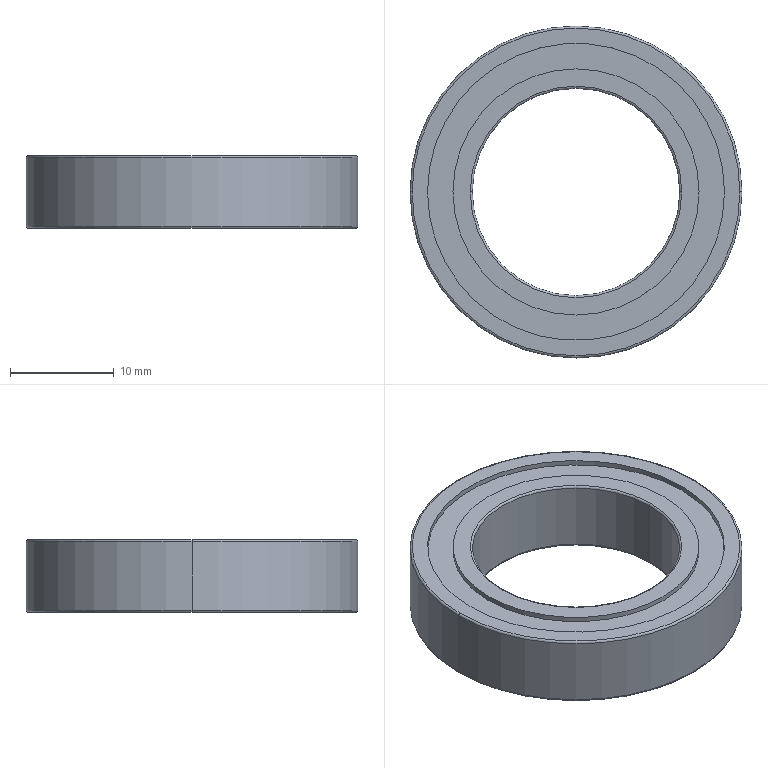Part | NX | features BREP 1 | 1 solid | 26 faces | box 32 x 32 x 7 mm | volume 3226 mm3 | cylinder 12 | torus 8 | plane 6 | commonest cylinder face diameters 23.732 x4 28.634 x4 20 x2 32 x2
STEP:
#1=CARTESIAN_POINT('',(-14.317,0.,3.));
#2=VERTEX_POINT('',#1);
#3=CARTESIAN_POINT('',(-14.317,0.,3.5));
#4=VERTEX_POINT('',#3);
#5=CARTESIAN_POINT('',(-14.317,0.,3.5));
#6=DIRECTION('',(0.,0.,-1.));
#7=VECTOR('',#6,1000.);
#8=LINE('',#5,#7);
#9=EDGE_CURVE('',#2,#4,#8,.F.);
#10=ORIENTED_EDGE('',*,*,#9,.T.);
#11=CARTESIAN_POINT('',(14.317,0.,3.5));
#12=VERTEX_POINT('',#11);
#13=CARTESIAN_POINT('',(0.,0.,3.5));
#14=DIRECTION('',(0.,0.,-1.));
#15=DIRECTION('',(1.,0.,0.));
#16=AXIS2_PLACEMENT_3D('',#13,#14,#15);
#17=CIRCLE('',#16,14.317);
#18=EDGE_CURVE('',#12,#4,#17,.T.);
#19=ORIENTED_EDGE('',*,*,#18,.F.);
#20=CARTESIAN_POINT('',(14.317,0.,3.));
#21=VERTEX_POINT('',#20);
#22=CARTESIAN_POINT('',(14.317,0.,3.5));
#23=DIRECTION('',(0.,0.,-1.));
#24=VECTOR('',#23,1000.);
#25=LINE('',#22,#24);
#26=EDGE_CURVE('',#21,#12,#25,.F.);
#27=ORIENTED_EDGE('',*,*,#26,.F.);
#28=CARTESIAN_POINT('',(0.,0.,3.));
#29=DIRECTION('',(0.,0.,1.));
#30=DIRECTION('',(-1.,0.,0.));
#31=AXIS2_PLACEMENT_3D('',#28,#29,#30);
#32=CIRCLE('',#31,14.317);
#33=EDGE_CURVE('',#2,#21,#32,.T.);
#34=ORIENTED_EDGE('',*,*,#33,.F.);
#35=EDGE_LOOP('',(#10,#19,#27,#34));
#36=FACE_BOUND('',#35,.T.);
#37=CARTESIAN_POINT('',(0.,0.,3.));
#38=DIRECTION('',(0.,0.,1.));
#39=DIRECTION('',(-1.,0.,0.));
#40=AXIS2_PLACEMENT_3D('',#37,#38,#39);
#41=CYLINDRICAL_SURFACE('',#40,14.317);
#42=ADVANCED_FACE('',(#36),#41,.F.);
#43=ORIENTED_EDGE('',*,*,#33,.T.);
#44=CARTESIAN_POINT('',(0.,0.,3.));
#45=DIRECTION('',(0.,0.,1.));
#46=DIRECTION('',(1.,0.,0.));
#47=AXIS2_PLACEMENT_3D('',#44,#45,#46);
#48=CIRCLE('',#47,14.317);
#49=EDGE_CURVE('',#21,#2,#48,.T.);
#50=ORIENTED_EDGE('',*,*,#49,.T.);
#51=EDGE_LOOP('',(#43,#50));
#52=FACE_BOUND('',#51,.T.);
#53=CARTESIAN_POINT('',(11.866,0.,3.));
#54=VERTEX_POINT('',#53);
#55=CARTESIAN_POINT('',(-11.866,0.,3.));
#56=VERTEX_POINT('',#55);
#57=CARTESIAN_POINT('',(0.,0.,3.));
#58=DIRECTION('',(0.,0.,-1.));
#59=DIRECTION('',(1.,0.,0.));
#60=AXIS2_PLACEMENT_3D('',#57,#58,#59);
#61=CIRCLE('',#60,11.866);
#62=EDGE_CURVE('',#54,#56,#61,.T.);
#63=ORIENTED_EDGE('',*,*,#62,.T.);
#64=CARTESIAN_POINT('',(0.,0.,3.));
#65=DIRECTION('',(0.,0.,-1.));
#66=DIRECTION('',(-1.,0.,0.));
#67=AXIS2_PLACEMENT_3D('',#64,#65,#66);
#68=CIRCLE('',#67,11.866);
#69=EDGE_CURVE('',#56,#54,#68,.T.);
#70=ORIENTED_EDGE('',*,*,#69,.T.);
#71=EDGE_LOOP('',(#63,#70));
#72=FACE_BOUND('',#71,.T.);
#73=CARTESIAN_POINT('',(0.,0.,3.));
#74=DIRECTION('',(0.,0.,1.));
#75=DIRECTION('',(-1.,0.,0.));
#76=AXIS2_PLACEMENT_3D('',#73,#74,#75);
#77=PLANE('',#76);
#78=ADVANCED_FACE('',(#52,#72),#77,.T.);
#79=ORIENTED_EDGE('',*,*,#49,.F.);
#80=ORIENTED_EDGE('',*,*,#26,.T.);
#81=CARTESIAN_POINT('',(0.,0.,3.5));
#82=DIRECTION('',(0.,0.,-1.));
#83=DIRECTION('',(-1.,0.,0.));
#84=AXIS2_PLACEMENT_3D('',#81,#82,#83);
#85=CIRCLE('',#84,14.317);
#86=EDGE_CURVE('',#4,#12,#85,.T.);
#87=ORIENTED_EDGE('',*,*,#86,.F.);
#88=ORIENTED_EDGE('',*,*,#9,.F.);
#89=EDGE_LOOP('',(#79,#80,#87,#88));
#90=FACE_BOUND('',#89,.T.);
#91=CARTESIAN_POINT('',(0.,0.,3.));
#92=DIRECTION('',(0.,0.,1.));
#93=DIRECTION('',(-1.,0.,0.));
#94=AXIS2_PLACEMENT_3D('',#91,#92,#93);
#95=CYLINDRICAL_SURFACE('',#94,14.317);
#96=ADVANCED_FACE('',(#90),#95,.F.);
#97=CARTESIAN_POINT('',(-15.8,0.,3.5));
#98=VERTEX_POINT('',#97);
#99=CARTESIAN_POINT('',(15.8,0.,3.5));
#100=VERTEX_POINT('',#99);
#101=CARTESIAN_POINT('',(0.,0.,3.5));
#102=DIRECTION('',(0.,0.,1.));
#103=DIRECTION('',(-1.,0.,0.));
#104=AXIS2_PLACEMENT_3D('',#101,#102,#103);
#105=CIRCLE('',#104,15.8);
#106=EDGE_CURVE('',#98,#100,#105,.T.);
#107=ORIENTED_EDGE('',*,*,#106,.T.);
#108=CARTESIAN_POINT('',(0.,0.,3.5));
#109=DIRECTION('',(0.,0.,1.));
#110=DIRECTION('',(1.,0.,0.));
#111=AXIS2_PLACEMENT_3D('',#108,#109,#110);
#112=CIRCLE('',#111,15.8);
#113=EDGE_CURVE('',#100,#98,#112,.T.);
#114=ORIENTED_EDGE('',*,*,#113,.T.);
#115=EDGE_LOOP('',(#107,#114));
#116=FACE_BOUND('',#115,.T.);
#117=ORIENTED_EDGE('',*,*,#18,.T.);
#118=ORIENTED_EDGE('',*,*,#86,.T.);
#119=EDGE_LOOP('',(#117,#118));
#120=FACE_BOUND('',#119,.T.);
#121=CARTESIAN_POINT('',(0.,0.,3.5));
#122=DIRECTION('',(0.,0.,1.));
#123=DIRECTION('',(-1.,0.,0.));
#124=AXIS2_PLACEMENT_3D('',#121,#122,#123);
#125=PLANE('',#124);
#126=ADVANCED_FACE('',(#116,#120),#125,.T.);
#127=CARTESIAN_POINT('',(-16.,0.,3.3));
#128=VERTEX_POINT('',#127);
#129=CARTESIAN_POINT('',(-15.8,0.,3.3));
#130=DIRECTION('',(0.,-1.,0.));
#131=DIRECTION('',(0.,0.,1.));
#132=AXIS2_PLACEMENT_3D('',#129,#130,#131);
#133=CIRCLE('',#132,0.2);
#134=EDGE_CURVE('',#128,#98,#133,.F.);
#135=ORIENTED_EDGE('',*,*,#134,.T.);
#136=ORIENTED_EDGE('',*,*,#113,.F.);
#137=CARTESIAN_POINT('',(16.,0.,3.3));
#138=VERTEX_POINT('',#137);
#139=CARTESIAN_POINT('',(15.8,0.,3.3));
#140=DIRECTION('',(0.,1.,0.));
#141=DIRECTION('',(0.,0.,1.));
#142=AXIS2_PLACEMENT_3D('',#139,#140,#141);
#143=CIRCLE('',#142,0.2);
#144=EDGE_CURVE('',#138,#100,#143,.F.);
#145=ORIENTED_EDGE('',*,*,#144,.F.);
#146=CARTESIAN_POINT('',(0.,0.,3.3));
#147=DIRECTION('',(0.,0.,1.));
#148=DIRECTION('',(1.,0.,0.));
#149=AXIS2_PLACEMENT_3D('',#146,#147,#148);
#150=CIRCLE('',#149,16.);
#151=EDGE_CURVE('',#138,#128,#150,.T.);
#152=ORIENTED_EDGE('',*,*,#151,.T.);
#153=EDGE_LOOP('',(#135,#136,#145,#152));
#154=FACE_BOUND('',#153,.T.);
#155=CARTESIAN_POINT('',(0.,0.,3.3));
#156=DIRECTION('',(0.,0.,1.));
#157=DIRECTION('',(-1.,0.,0.));
#158=AXIS2_PLACEMENT_3D('',#155,#156,#157);
#159=TOROIDAL_SURFACE('',#158,15.8,0.2);
#160=ADVANCED_FACE('',(#154),#159,.T.);
#161=CARTESIAN_POINT('',(16.,0.,-3.3));
#162=VERTEX_POINT('',#161);
#163=CARTESIAN_POINT('',(16.,0.,-3.3));
#164=DIRECTION('',(0.,0.,1.));
#165=VECTOR('',#164,1000.);
#166=LINE('',#163,#165);
#167=EDGE_CURVE('',#162,#138,#166,.T.);
#168=ORIENTED_EDGE('',*,*,#167,.F.);
#169=CARTESIAN_POINT('',(-16.,0.,-3.3));
#170=VERTEX_POINT('',#169);
#171=CARTESIAN_POINT('',(0.,0.,-3.3));
#172=DIRECTION('',(0.,0.,-1.));
#173=DIRECTION('',(-1.,0.,0.));
#174=AXIS2_PLACEMENT_3D('',#171,#172,#173);
#175=CIRCLE('',#174,16.);
#176=EDGE_CURVE('',#170,#162,#175,.T.);
#177=ORIENTED_EDGE('',*,*,#176,.F.);
#178=CARTESIAN_POINT('',(-16.,0.,-3.3));
#179=DIRECTION('',(0.,0.,1.));
#180=VECTOR('',#179,1000.);
#181=LINE('',#178,#180);
#182=EDGE_CURVE('',#170,#128,#181,.T.);
#183=ORIENTED_EDGE('',*,*,#182,.T.);
#184=ORIENTED_EDGE('',*,*,#151,.F.);
#185=EDGE_LOOP('',(#168,#177,#183,#184));
#186=FACE_BOUND('',#185,.T.);
#187=CARTESIAN_POINT('',(0.,0.,3.5));
#188=DIRECTION('',(0.,0.,-1.));
#189=DIRECTION('',(1.,0.,0.));
#190=AXIS2_PLACEMENT_3D('',#187,#188,#189);
#191=CYLINDRICAL_SURFACE('',#190,16.);
#192=ADVANCED_FACE('',(#186),#191,.T.);
#193=CARTESIAN_POINT('',(0.,0.,3.3));
#194=DIRECTION('',(0.,0.,1.));
#195=DIRECTION('',(-1.,0.,0.));
#196=AXIS2_PLACEMENT_3D('',#193,#194,#195);
#197=CIRCLE('',#196,16.);
#198=EDGE_CURVE('',#128,#138,#197,.T.);
#199=ORIENTED_EDGE('',*,*,#198,.F.);
#200=ORIENTED_EDGE('',*,*,#182,.F.);
#201=CARTESIAN_POINT('',(0.,0.,-3.3));
#202=DIRECTION('',(0.,0.,-1.));
#203=DIRECTION('',(1.,0.,0.));
#204=AXIS2_PLACEMENT_3D('',#201,#202,#203);
#205=CIRCLE('',#204,16.);
#206=EDGE_CURVE('',#162,#170,#205,.T.);
#207=ORIENTED_EDGE('',*,*,#206,.F.);
#208=ORIENTED_EDGE('',*,*,#167,.T.);
#209=EDGE_LOOP('',(#199,#200,#207,#208));
#210=FACE_BOUND('',#209,.T.);
#211=CARTESIAN_POINT('',(0.,0.,3.5));
#212=DIRECTION('',(0.,0.,-1.));
#213=DIRECTION('',(1.,0.,0.));
#214=AXIS2_PLACEMENT_3D('',#211,#212,#213);
#215=CYLINDRICAL_SURFACE('',#214,16.);
#216=ADVANCED_FACE('',(#210),#215,.T.);
#217=CARTESIAN_POINT('',(15.8,0.,-3.5));
#218=VERTEX_POINT('',#217);
#219=CARTESIAN_POINT('',(-15.8,0.,-3.5));
#220=VERTEX_POINT('',#219);
#221=CARTESIAN_POINT('',(0.,0.,-3.5));
#222=DIRECTION('',(0.,0.,-1.));
#223=DIRECTION('',(1.,0.,0.));
#224=AXIS2_PLACEMENT_3D('',#221,#222,#223);
#225=CIRCLE('',#224,15.8);
#226=EDGE_CURVE('',#218,#220,#225,.T.);
#227=ORIENTED_EDGE('',*,*,#226,.F.);
#228=CARTESIAN_POINT('',(15.8,0.,-3.3));
#229=DIRECTION('',(0.,1.,0.));
#230=DIRECTION('',(1.,0.,0.));
#231=AXIS2_PLACEMENT_3D('',#228,#229,#230);
#232=CIRCLE('',#231,0.2);
#233=EDGE_CURVE('',#162,#218,#232,.T.);
#234=ORIENTED_EDGE('',*,*,#233,.F.);
#235=ORIENTED_EDGE('',*,*,#206,.T.);
#236=CARTESIAN_POINT('',(-15.8,0.,-3.3));
#237=DIRECTION('',(0.,-1.,0.));
#238=DIRECTION('',(-1.,0.,0.));
#239=AXIS2_PLACEMENT_3D('',#236,#237,#238);
#240=CIRCLE('',#239,0.2);
#241=EDGE_CURVE('',#170,#220,#240,.T.);
#242=ORIENTED_EDGE('',*,*,#241,.T.);
#243=EDGE_LOOP('',(#227,#234,#235,#242));
#244=FACE_BOUND('',#243,.T.);
#245=CARTESIAN_POINT('',(0.,0.,-3.3));
#246=DIRECTION('',(0.,0.,1.));
#247=DIRECTION('',(-1.,0.,0.));
#248=AXIS2_PLACEMENT_3D('',#245,#246,#247);
#249=TOROIDAL_SURFACE('',#248,15.8,0.2);
#250=ADVANCED_FACE('',(#244),#249,.T.);
#251=ORIENTED_EDGE('',*,*,#241,.F.);
#252=ORIENTED_EDGE('',*,*,#176,.T.);
#253=ORIENTED_EDGE('',*,*,#233,.T.);
#254=CARTESIAN_POINT('',(0.,0.,-3.5));
#255=DIRECTION('',(0.,0.,-1.));
#256=DIRECTION('',(-1.,0.,0.));
#257=AXIS2_PLACEMENT_3D('',#254,#255,#256);
#258=CIRCLE('',#257,15.8);
#259=EDGE_CURVE('',#220,#218,#258,.T.);
#260=ORIENTED_EDGE('',*,*,#259,.F.);
#261=EDGE_LOOP('',(#251,#252,#253,#260));
#262=FACE_BOUND('',#261,.T.);
#263=CARTESIAN_POINT('',(0.,0.,-3.3));
#264=DIRECTION('',(0.,0.,1.));
#265=DIRECTION('',(-1.,0.,0.));
#266=AXIS2_PLACEMENT_3D('',#263,#264,#265);
#267=TOROIDAL_SURFACE('',#266,15.8,0.2);
#268=ADVANCED_FACE('',(#262),#267,.T.);
#269=ORIENTED_EDGE('',*,*,#259,.T.);
#270=ORIENTED_EDGE('',*,*,#226,.T.);
#271=EDGE_LOOP('',(#269,#270));
#272=FACE_BOUND('',#271,.T.);
#273=CARTESIAN_POINT('',(14.317,0.,-3.5));
#274=VERTEX_POINT('',#273);
#275=CARTESIAN_POINT('',(-14.317,0.,-3.5));
#276=VERTEX_POINT('',#275);
#277=CARTESIAN_POINT('',(0.,0.,-3.5));
#278=DIRECTION('',(0.,0.,1.));
#279=DIRECTION('',(1.,0.,0.));
#280=AXIS2_PLACEMENT_3D('',#277,#278,#279);
#281=CIRCLE('',#280,14.317);
#282=EDGE_CURVE('',#274,#276,#281,.T.);
#283=ORIENTED_EDGE('',*,*,#282,.T.);
#284=CARTESIAN_POINT('',(0.,0.,-3.5));
#285=DIRECTION('',(0.,0.,1.));
#286=DIRECTION('',(-1.,0.,0.));
#287=AXIS2_PLACEMENT_3D('',#284,#285,#286);
#288=CIRCLE('',#287,14.317);
#289=EDGE_CURVE('',#276,#274,#288,.T.);
#290=ORIENTED_EDGE('',*,*,#289,.T.);
#291=EDGE_LOOP('',(#283,#290));
#292=FACE_BOUND('',#291,.T.);
#293=CARTESIAN_POINT('',(0.,0.,-3.5));
#294=DIRECTION('',(0.,0.,1.));
#295=DIRECTION('',(-1.,0.,0.));
#296=AXIS2_PLACEMENT_3D('',#293,#294,#295);
#297=PLANE('',#296);
#298=ADVANCED_FACE('',(#272,#292),#297,.F.);
#299=CARTESIAN_POINT('',(14.317,0.,-3.));
#300=VERTEX_POINT('',#299);
#301=CARTESIAN_POINT('',(14.317,0.,-3.5));
#302=DIRECTION('',(0.,0.,1.));
#303=VECTOR('',#302,1000.);
#304=LINE('',#301,#303);
#305=EDGE_CURVE('',#274,#300,#304,.T.);
#306=ORIENTED_EDGE('',*,*,#305,.F.);
#307=ORIENTED_EDGE('',*,*,#289,.F.);
#308=CARTESIAN_POINT('',(-14.317,0.,-3.));
#309=VERTEX_POINT('',#308);
#310=CARTESIAN_POINT('',(-14.317,0.,-3.5));
#311=DIRECTION('',(0.,0.,1.));
#312=VECTOR('',#311,1000.);
#313=LINE('',#310,#312);
#314=EDGE_CURVE('',#276,#309,#313,.T.);
#315=ORIENTED_EDGE('',*,*,#314,.T.);
#316=CARTESIAN_POINT('',(0.,0.,-3.));
#317=DIRECTION('',(0.,0.,-1.));
#318=DIRECTION('',(1.,0.,0.));
#319=AXIS2_PLACEMENT_3D('',#316,#317,#318);
#320=CIRCLE('',#319,14.317);
#321=EDGE_CURVE('',#300,#309,#320,.T.);
#322=ORIENTED_EDGE('',*,*,#321,.F.);
#323=EDGE_LOOP('',(#306,#307,#315,#322));
#324=FACE_BOUND('',#323,.T.);
#325=CARTESIAN_POINT('',(0.,0.,-3.));
#326=DIRECTION('',(0.,0.,-1.));
#327=DIRECTION('',(1.,0.,0.));
#328=AXIS2_PLACEMENT_3D('',#325,#326,#327);
#329=CYLINDRICAL_SURFACE('',#328,14.317);
#330=ADVANCED_FACE('',(#324),#329,.F.);
#331=CARTESIAN_POINT('',(0.,0.,-3.));
#332=DIRECTION('',(0.,0.,-1.));
#333=DIRECTION('',(-1.,0.,0.));
#334=AXIS2_PLACEMENT_3D('',#331,#332,#333);
#335=CIRCLE('',#334,14.317);
#336=EDGE_CURVE('',#309,#300,#335,.T.);
#337=ORIENTED_EDGE('',*,*,#336,.T.);
#338=ORIENTED_EDGE('',*,*,#321,.T.);
#339=EDGE_LOOP('',(#337,#338));
#340=FACE_BOUND('',#339,.T.);
#341=CARTESIAN_POINT('',(11.866,0.,-3.));
#342=VERTEX_POINT('',#341);
#343=CARTESIAN_POINT('',(-11.866,0.,-3.));
#344=VERTEX_POINT('',#343);
#345=CARTESIAN_POINT('',(0.,0.,-3.));
#346=DIRECTION('',(0.,0.,1.));
#347=DIRECTION('',(1.,0.,0.));
#348=AXIS2_PLACEMENT_3D('',#345,#346,#347);
#349=CIRCLE('',#348,11.866);
#350=EDGE_CURVE('',#342,#344,#349,.T.);
#351=ORIENTED_EDGE('',*,*,#350,.T.);
#352=CARTESIAN_POINT('',(0.,0.,-3.));
#353=DIRECTION('',(0.,0.,1.));
#354=DIRECTION('',(-1.,0.,0.));
#355=AXIS2_PLACEMENT_3D('',#352,#353,#354);
#356=CIRCLE('',#355,11.866);
#357=EDGE_CURVE('',#344,#342,#356,.T.);
#358=ORIENTED_EDGE('',*,*,#357,.T.);
#359=EDGE_LOOP('',(#351,#358));
#360=FACE_BOUND('',#359,.T.);
#361=CARTESIAN_POINT('',(0.,0.,-3.));
#362=DIRECTION('',(0.,0.,-1.));
#363=DIRECTION('',(-1.,0.,0.));
#364=AXIS2_PLACEMENT_3D('',#361,#362,#363);
#365=PLANE('',#364);
#366=ADVANCED_FACE('',(#340,#360),#365,.T.);
#367=ORIENTED_EDGE('',*,*,#336,.F.);
#368=ORIENTED_EDGE('',*,*,#314,.F.);
#369=ORIENTED_EDGE('',*,*,#282,.F.);
#370=ORIENTED_EDGE('',*,*,#305,.T.);
#371=EDGE_LOOP('',(#367,#368,#369,#370));
#372=FACE_BOUND('',#371,.T.);
#373=CARTESIAN_POINT('',(0.,0.,-3.));
#374=DIRECTION('',(0.,0.,-1.));
#375=DIRECTION('',(1.,0.,0.));
#376=AXIS2_PLACEMENT_3D('',#373,#374,#375);
#377=CYLINDRICAL_SURFACE('',#376,14.317);
#378=ADVANCED_FACE('',(#372),#377,.F.);
#379=ORIENTED_EDGE('',*,*,#357,.F.);
#380=CARTESIAN_POINT('',(-11.866,0.,-3.5));
#381=VERTEX_POINT('',#380);
#382=CARTESIAN_POINT('',(-11.866,0.,-3.5));
#383=DIRECTION('',(0.,0.,1.));
#384=VECTOR('',#383,1000.);
#385=LINE('',#382,#384);
#386=EDGE_CURVE('',#344,#381,#385,.F.);
#387=ORIENTED_EDGE('',*,*,#386,.T.);
#388=CARTESIAN_POINT('',(11.866,0.,-3.5));
#389=VERTEX_POINT('',#388);
#390=CARTESIAN_POINT('',(0.,0.,-3.5));
#391=DIRECTION('',(0.,0.,-1.));
#392=DIRECTION('',(1.,0.,0.));
#393=AXIS2_PLACEMENT_3D('',#390,#391,#392);
#394=CIRCLE('',#393,11.866);
#395=EDGE_CURVE('',#389,#381,#394,.T.);
#396=ORIENTED_EDGE('',*,*,#395,.F.);
#397=CARTESIAN_POINT('',(11.866,0.,-3.5));
#398=DIRECTION('',(0.,0.,1.));
#399=VECTOR('',#398,1000.);
#400=LINE('',#397,#399);
#401=EDGE_CURVE('',#342,#389,#400,.F.);
#402=ORIENTED_EDGE('',*,*,#401,.F.);
#403=EDGE_LOOP('',(#379,#387,#396,#402));
#404=FACE_BOUND('',#403,.T.);
#405=CARTESIAN_POINT('',(0.,0.,-3.));
#406=DIRECTION('',(0.,0.,-1.));
#407=DIRECTION('',(1.,0.,0.));
#408=AXIS2_PLACEMENT_3D('',#405,#406,#407);
#409=CYLINDRICAL_SURFACE('',#408,11.866);
#410=ADVANCED_FACE('',(#404),#409,.T.);
#411=ORIENTED_EDGE('',*,*,#401,.T.);
#412=CARTESIAN_POINT('',(0.,0.,-3.5));
#413=DIRECTION('',(0.,0.,-1.));
#414=DIRECTION('',(-1.,0.,0.));
#415=AXIS2_PLACEMENT_3D('',#412,#413,#414);
#416=CIRCLE('',#415,11.866);
#417=EDGE_CURVE('',#381,#389,#416,.T.);
#418=ORIENTED_EDGE('',*,*,#417,.F.);
#419=ORIENTED_EDGE('',*,*,#386,.F.);
#420=ORIENTED_EDGE('',*,*,#350,.F.);
#421=EDGE_LOOP('',(#411,#418,#419,#420));
#422=FACE_BOUND('',#421,.T.);
#423=CARTESIAN_POINT('',(0.,0.,-3.));
#424=DIRECTION('',(0.,0.,-1.));
#425=DIRECTION('',(1.,0.,0.));
#426=AXIS2_PLACEMENT_3D('',#423,#424,#425);
#427=CYLINDRICAL_SURFACE('',#426,11.866);
#428=ADVANCED_FACE('',(#422),#427,.T.);
#429=ORIENTED_EDGE('',*,*,#417,.T.);
#430=ORIENTED_EDGE('',*,*,#395,.T.);
#431=EDGE_LOOP('',(#429,#430));
#432=FACE_BOUND('',#431,.T.);
#433=CARTESIAN_POINT('',(-10.2,0.,-3.5));
#434=VERTEX_POINT('',#433);
#435=CARTESIAN_POINT('',(10.2,0.,-3.5));
#436=VERTEX_POINT('',#435);
#437=CARTESIAN_POINT('',(0.,0.,-3.5));
#438=DIRECTION('',(0.,0.,1.));
#439=DIRECTION('',(-1.,0.,0.));
#440=AXIS2_PLACEMENT_3D('',#437,#438,#439);
#441=CIRCLE('',#440,10.2);
#442=EDGE_CURVE('',#434,#436,#441,.T.);
#443=ORIENTED_EDGE('',*,*,#442,.T.);
#444=CARTESIAN_POINT('',(0.,0.,-3.5));
#445=DIRECTION('',(0.,0.,1.));
#446=DIRECTION('',(1.,0.,0.));
#447=AXIS2_PLACEMENT_3D('',#444,#445,#446);
#448=CIRCLE('',#447,10.2);
#449=EDGE_CURVE('',#436,#434,#448,.T.);
#450=ORIENTED_EDGE('',*,*,#449,.T.);
#451=EDGE_LOOP('',(#443,#450));
#452=FACE_BOUND('',#451,.T.);
#453=CARTESIAN_POINT('',(0.,0.,-3.5));
#454=DIRECTION('',(0.,0.,1.));
#455=DIRECTION('',(-1.,0.,0.));
#456=AXIS2_PLACEMENT_3D('',#453,#454,#455);
#457=PLANE('',#456);
#458=ADVANCED_FACE('',(#432,#452),#457,.F.);
#459=CARTESIAN_POINT('',(-10.,0.,-3.3));
#460=VERTEX_POINT('',#459);
#461=CARTESIAN_POINT('',(-10.2,0.,-3.3));
#462=DIRECTION('',(0.,-1.,0.));
#463=DIRECTION('',(0.,0.,-1.));
#464=AXIS2_PLACEMENT_3D('',#461,#462,#463);
#465=CIRCLE('',#464,0.2);
#466=EDGE_CURVE('',#460,#434,#465,.F.);
#467=ORIENTED_EDGE('',*,*,#466,.T.);
#468=ORIENTED_EDGE('',*,*,#449,.F.);
#469=CARTESIAN_POINT('',(10.,0.,-3.3));
#470=VERTEX_POINT('',#469);
#471=CARTESIAN_POINT('',(10.2,0.,-3.3));
#472=DIRECTION('',(0.,1.,0.));
#473=DIRECTION('',(0.,0.,-1.));
#474=AXIS2_PLACEMENT_3D('',#471,#472,#473);
#475=CIRCLE('',#474,0.2);
#476=EDGE_CURVE('',#470,#436,#475,.F.);
#477=ORIENTED_EDGE('',*,*,#476,.F.);
#478=CARTESIAN_POINT('',(0.,0.,-3.3));
#479=DIRECTION('',(0.,0.,1.));
#480=DIRECTION('',(1.,0.,0.));
#481=AXIS2_PLACEMENT_3D('',#478,#479,#480);
#482=CIRCLE('',#481,10.);
#483=EDGE_CURVE('',#470,#460,#482,.T.);
#484=ORIENTED_EDGE('',*,*,#483,.T.);
#485=EDGE_LOOP('',(#467,#468,#477,#484));
#486=FACE_BOUND('',#485,.T.);
#487=CARTESIAN_POINT('',(0.,0.,-3.3));
#488=DIRECTION('',(0.,0.,1.));
#489=DIRECTION('',(-1.,0.,0.));
#490=AXIS2_PLACEMENT_3D('',#487,#488,#489);
#491=TOROIDAL_SURFACE('',#490,10.2,0.2);
#492=ADVANCED_FACE('',(#486),#491,.T.);
#493=CARTESIAN_POINT('',(-10.,0.,3.3));
#494=VERTEX_POINT('',#493);
#495=CARTESIAN_POINT('',(10.,0.,3.3));
#496=VERTEX_POINT('',#495);
#497=CARTESIAN_POINT('',(0.,0.,3.3));
#498=DIRECTION('',(0.,0.,-1.));
#499=DIRECTION('',(-1.,0.,0.));
#500=AXIS2_PLACEMENT_3D('',#497,#498,#499);
#501=CIRCLE('',#500,10.);
#502=EDGE_CURVE('',#494,#496,#501,.T.);
#503=ORIENTED_EDGE('',*,*,#502,.F.);
#504=CARTESIAN_POINT('',(-10.,0.,-3.3));
#505=DIRECTION('',(0.,0.,1.));
#506=VECTOR('',#505,1000.);
#507=LINE('',#504,#506);
#508=EDGE_CURVE('',#494,#460,#507,.F.);
#509=ORIENTED_EDGE('',*,*,#508,.T.);
#510=ORIENTED_EDGE('',*,*,#483,.F.);
#511=CARTESIAN_POINT('',(10.,0.,-3.3));
#512=DIRECTION('',(0.,0.,1.));
#513=VECTOR('',#512,1000.);
#514=LINE('',#511,#513);
#515=EDGE_CURVE('',#496,#470,#514,.F.);
#516=ORIENTED_EDGE('',*,*,#515,.F.);
#517=EDGE_LOOP('',(#503,#509,#510,#516));
#518=FACE_BOUND('',#517,.T.);
#519=CARTESIAN_POINT('',(0.,0.,3.5));
#520=DIRECTION('',(0.,0.,-1.));
#521=DIRECTION('',(1.,0.,0.));
#522=AXIS2_PLACEMENT_3D('',#519,#520,#521);
#523=CYLINDRICAL_SURFACE('',#522,10.);
#524=ADVANCED_FACE('',(#518),#523,.F.);
#525=ORIENTED_EDGE('',*,*,#515,.T.);
#526=CARTESIAN_POINT('',(0.,0.,-3.3));
#527=DIRECTION('',(0.,0.,1.));
#528=DIRECTION('',(-1.,0.,0.));
#529=AXIS2_PLACEMENT_3D('',#526,#527,#528);
#530=CIRCLE('',#529,10.);
#531=EDGE_CURVE('',#460,#470,#530,.T.);
#532=ORIENTED_EDGE('',*,*,#531,.F.);
#533=ORIENTED_EDGE('',*,*,#508,.F.);
#534=CARTESIAN_POINT('',(0.,0.,3.3));
#535=DIRECTION('',(0.,0.,-1.));
#536=DIRECTION('',(1.,0.,0.));
#537=AXIS2_PLACEMENT_3D('',#534,#535,#536);
#538=CIRCLE('',#537,10.);
#539=EDGE_CURVE('',#496,#494,#538,.T.);
#540=ORIENTED_EDGE('',*,*,#539,.F.);
#541=EDGE_LOOP('',(#525,#532,#533,#540));
#542=FACE_BOUND('',#541,.T.);
#543=CARTESIAN_POINT('',(0.,0.,3.5));
#544=DIRECTION('',(0.,0.,-1.));
#545=DIRECTION('',(1.,0.,0.));
#546=AXIS2_PLACEMENT_3D('',#543,#544,#545);
#547=CYLINDRICAL_SURFACE('',#546,10.);
#548=ADVANCED_FACE('',(#542),#547,.F.);
#549=CARTESIAN_POINT('',(10.2,0.,3.5));
#550=VERTEX_POINT('',#549);
#551=CARTESIAN_POINT('',(-10.2,0.,3.5));
#552=VERTEX_POINT('',#551);
#553=CARTESIAN_POINT('',(0.,0.,3.5));
#554=DIRECTION('',(0.,0.,-1.));
#555=DIRECTION('',(1.,0.,0.));
#556=AXIS2_PLACEMENT_3D('',#553,#554,#555);
#557=CIRCLE('',#556,10.2);
#558=EDGE_CURVE('',#550,#552,#557,.T.);
#559=ORIENTED_EDGE('',*,*,#558,.F.);
#560=CARTESIAN_POINT('',(10.2,0.,3.3));
#561=DIRECTION('',(0.,1.,0.));
#562=DIRECTION('',(-1.,0.,0.));
#563=AXIS2_PLACEMENT_3D('',#560,#561,#562);
#564=CIRCLE('',#563,0.2);
#565=EDGE_CURVE('',#496,#550,#564,.T.);
#566=ORIENTED_EDGE('',*,*,#565,.F.);
#567=ORIENTED_EDGE('',*,*,#539,.T.);
#568=CARTESIAN_POINT('',(-10.2,0.,3.3));
#569=DIRECTION('',(0.,-1.,0.));
#570=DIRECTION('',(1.,0.,0.));
#571=AXIS2_PLACEMENT_3D('',#568,#569,#570);
#572=CIRCLE('',#571,0.2);
#573=EDGE_CURVE('',#494,#552,#572,.T.);
#574=ORIENTED_EDGE('',*,*,#573,.T.);
#575=EDGE_LOOP('',(#559,#566,#567,#574));
#576=FACE_BOUND('',#575,.T.);
#577=CARTESIAN_POINT('',(0.,0.,3.3));
#578=DIRECTION('',(0.,0.,1.));
#579=DIRECTION('',(-1.,0.,0.));
#580=AXIS2_PLACEMENT_3D('',#577,#578,#579);
#581=TOROIDAL_SURFACE('',#580,10.2,0.2);
#582=ADVANCED_FACE('',(#576),#581,.T.);
#583=ORIENTED_EDGE('',*,*,#573,.F.);
#584=ORIENTED_EDGE('',*,*,#502,.T.);
#585=ORIENTED_EDGE('',*,*,#565,.T.);
#586=CARTESIAN_POINT('',(0.,0.,3.5));
#587=DIRECTION('',(0.,0.,-1.));
#588=DIRECTION('',(-1.,0.,0.));
#589=AXIS2_PLACEMENT_3D('',#586,#587,#588);
#590=CIRCLE('',#589,10.2);
#591=EDGE_CURVE('',#552,#550,#590,.T.);
#592=ORIENTED_EDGE('',*,*,#591,.F.);
#593=EDGE_LOOP('',(#583,#584,#585,#592));
#594=FACE_BOUND('',#593,.T.);
#595=CARTESIAN_POINT('',(0.,0.,3.3));
#596=DIRECTION('',(0.,0.,1.));
#597=DIRECTION('',(-1.,0.,0.));
#598=AXIS2_PLACEMENT_3D('',#595,#596,#597);
#599=TOROIDAL_SURFACE('',#598,10.2,0.2);
#600=ADVANCED_FACE('',(#594),#599,.T.);
#601=CARTESIAN_POINT('',(-11.866,0.,3.5));
#602=VERTEX_POINT('',#601);
#603=CARTESIAN_POINT('',(11.866,0.,3.5));
#604=VERTEX_POINT('',#603);
#605=CARTESIAN_POINT('',(0.,0.,3.5));
#606=DIRECTION('',(0.,0.,1.));
#607=DIRECTION('',(-1.,0.,0.));
#608=AXIS2_PLACEMENT_3D('',#605,#606,#607);
#609=CIRCLE('',#608,11.866);
#610=EDGE_CURVE('',#602,#604,#609,.T.);
#611=ORIENTED_EDGE('',*,*,#610,.T.);
#612=CARTESIAN_POINT('',(0.,0.,3.5));
#613=DIRECTION('',(0.,0.,1.));
#614=DIRECTION('',(1.,0.,0.));
#615=AXIS2_PLACEMENT_3D('',#612,#613,#614);
#616=CIRCLE('',#615,11.866);
#617=EDGE_CURVE('',#604,#602,#616,.T.);
#618=ORIENTED_EDGE('',*,*,#617,.T.);
#619=EDGE_LOOP('',(#611,#618));
#620=FACE_BOUND('',#619,.T.);
#621=ORIENTED_EDGE('',*,*,#591,.T.);
#622=ORIENTED_EDGE('',*,*,#558,.T.);
#623=EDGE_LOOP('',(#621,#622));
#624=FACE_BOUND('',#623,.T.);
#625=CARTESIAN_POINT('',(0.,0.,3.5));
#626=DIRECTION('',(0.,0.,1.));
#627=DIRECTION('',(-1.,0.,0.));
#628=AXIS2_PLACEMENT_3D('',#625,#626,#627);
#629=PLANE('',#628);
#630=ADVANCED_FACE('',(#620,#624),#629,.T.);
#631=CARTESIAN_POINT('',(-11.866,0.,3.5));
#632=DIRECTION('',(0.,0.,-1.));
#633=VECTOR('',#632,1000.);
#634=LINE('',#631,#633);
#635=EDGE_CURVE('',#56,#602,#634,.F.);
#636=ORIENTED_EDGE('',*,*,#635,.T.);
#637=ORIENTED_EDGE('',*,*,#617,.F.);
#638=CARTESIAN_POINT('',(11.866,0.,3.5));
#639=DIRECTION('',(0.,0.,-1.));
#640=VECTOR('',#639,1000.);
#641=LINE('',#638,#640);
#642=EDGE_CURVE('',#54,#604,#641,.F.);
#643=ORIENTED_EDGE('',*,*,#642,.F.);
#644=ORIENTED_EDGE('',*,*,#69,.F.);
#645=EDGE_LOOP('',(#636,#637,#643,#644));
#646=FACE_BOUND('',#645,.T.);
#647=CARTESIAN_POINT('',(0.,0.,3.));
#648=DIRECTION('',(0.,0.,1.));
#649=DIRECTION('',(-1.,0.,0.));
#650=AXIS2_PLACEMENT_3D('',#647,#648,#649);
#651=CYLINDRICAL_SURFACE('',#650,11.866);
#652=ADVANCED_FACE('',(#646),#651,.T.);
#653=ORIENTED_EDGE('',*,*,#62,.F.);
#654=ORIENTED_EDGE('',*,*,#642,.T.);
#655=ORIENTED_EDGE('',*,*,#610,.F.);
#656=ORIENTED_EDGE('',*,*,#635,.F.);
#657=EDGE_LOOP('',(#653,#654,#655,#656));
#658=FACE_BOUND('',#657,.T.);
#659=CARTESIAN_POINT('',(0.,0.,3.));
#660=DIRECTION('',(0.,0.,1.));
#661=DIRECTION('',(-1.,0.,0.));
#662=AXIS2_PLACEMENT_3D('',#659,#660,#661);
#663=CYLINDRICAL_SURFACE('',#662,11.866);
#664=ADVANCED_FACE('',(#658),#663,.T.);
#665=ORIENTED_EDGE('',*,*,#531,.T.);
#666=ORIENTED_EDGE('',*,*,#476,.T.);
#667=ORIENTED_EDGE('',*,*,#442,.F.);
#668=ORIENTED_EDGE('',*,*,#466,.F.);
#669=EDGE_LOOP('',(#665,#666,#667,#668));
#670=FACE_BOUND('',#669,.T.);
#671=CARTESIAN_POINT('',(0.,0.,-3.3));
#672=DIRECTION('',(0.,0.,1.));
#673=DIRECTION('',(-1.,0.,0.));
#674=AXIS2_PLACEMENT_3D('',#671,#672,#673);
#675=TOROIDAL_SURFACE('',#674,10.2,0.2);
#676=ADVANCED_FACE('',(#670),#675,.T.);
#677=ORIENTED_EDGE('',*,*,#198,.T.);
#678=ORIENTED_EDGE('',*,*,#144,.T.);
#679=ORIENTED_EDGE('',*,*,#106,.F.);
#680=ORIENTED_EDGE('',*,*,#134,.F.);
#681=EDGE_LOOP('',(#677,#678,#679,#680));
#682=FACE_BOUND('',#681,.T.);
#683=CARTESIAN_POINT('',(0.,0.,3.3));
#684=DIRECTION('',(0.,0.,1.));
#685=DIRECTION('',(-1.,0.,0.));
#686=AXIS2_PLACEMENT_3D('',#683,#684,#685);
#687=TOROIDAL_SURFACE('',#686,15.8,0.2);
#688=ADVANCED_FACE('',(#682),#687,.T.);
#689=CLOSED_SHELL('',(#42,#78,#96,#126,#160,#192,#216,#250,#268,#298,#330,#366,#378,#410,#428,#458,#492,#524,#548,#582,#600,#630,#652,#664,#676,#688));
#690=MANIFOLD_SOLID_BREP('',#689);
#691=(LENGTH_UNIT()NAMED_UNIT(*)SI_UNIT(.MILLI.,.METRE.));
#692=UNCERTAINTY_MEASURE_WITH_UNIT(LENGTH_MEASURE(0.00001),#691,'','');
#693=(NAMED_UNIT(*)PLANE_ANGLE_UNIT()SI_UNIT($,.RADIAN.));
#694=(NAMED_UNIT(*)SI_UNIT($,.STERADIAN.)SOLID_ANGLE_UNIT());
#695=(GEOMETRIC_REPRESENTATION_CONTEXT(3)GLOBAL_UNCERTAINTY_ASSIGNED_CONTEXT((#692))GLOBAL_UNIT_ASSIGNED_CONTEXT((#691,#693,#694))REPRESENTATION_CONTEXT('',''));
#696=ADVANCED_BREP_SHAPE_REPRESENTATION('',(#690),#695);